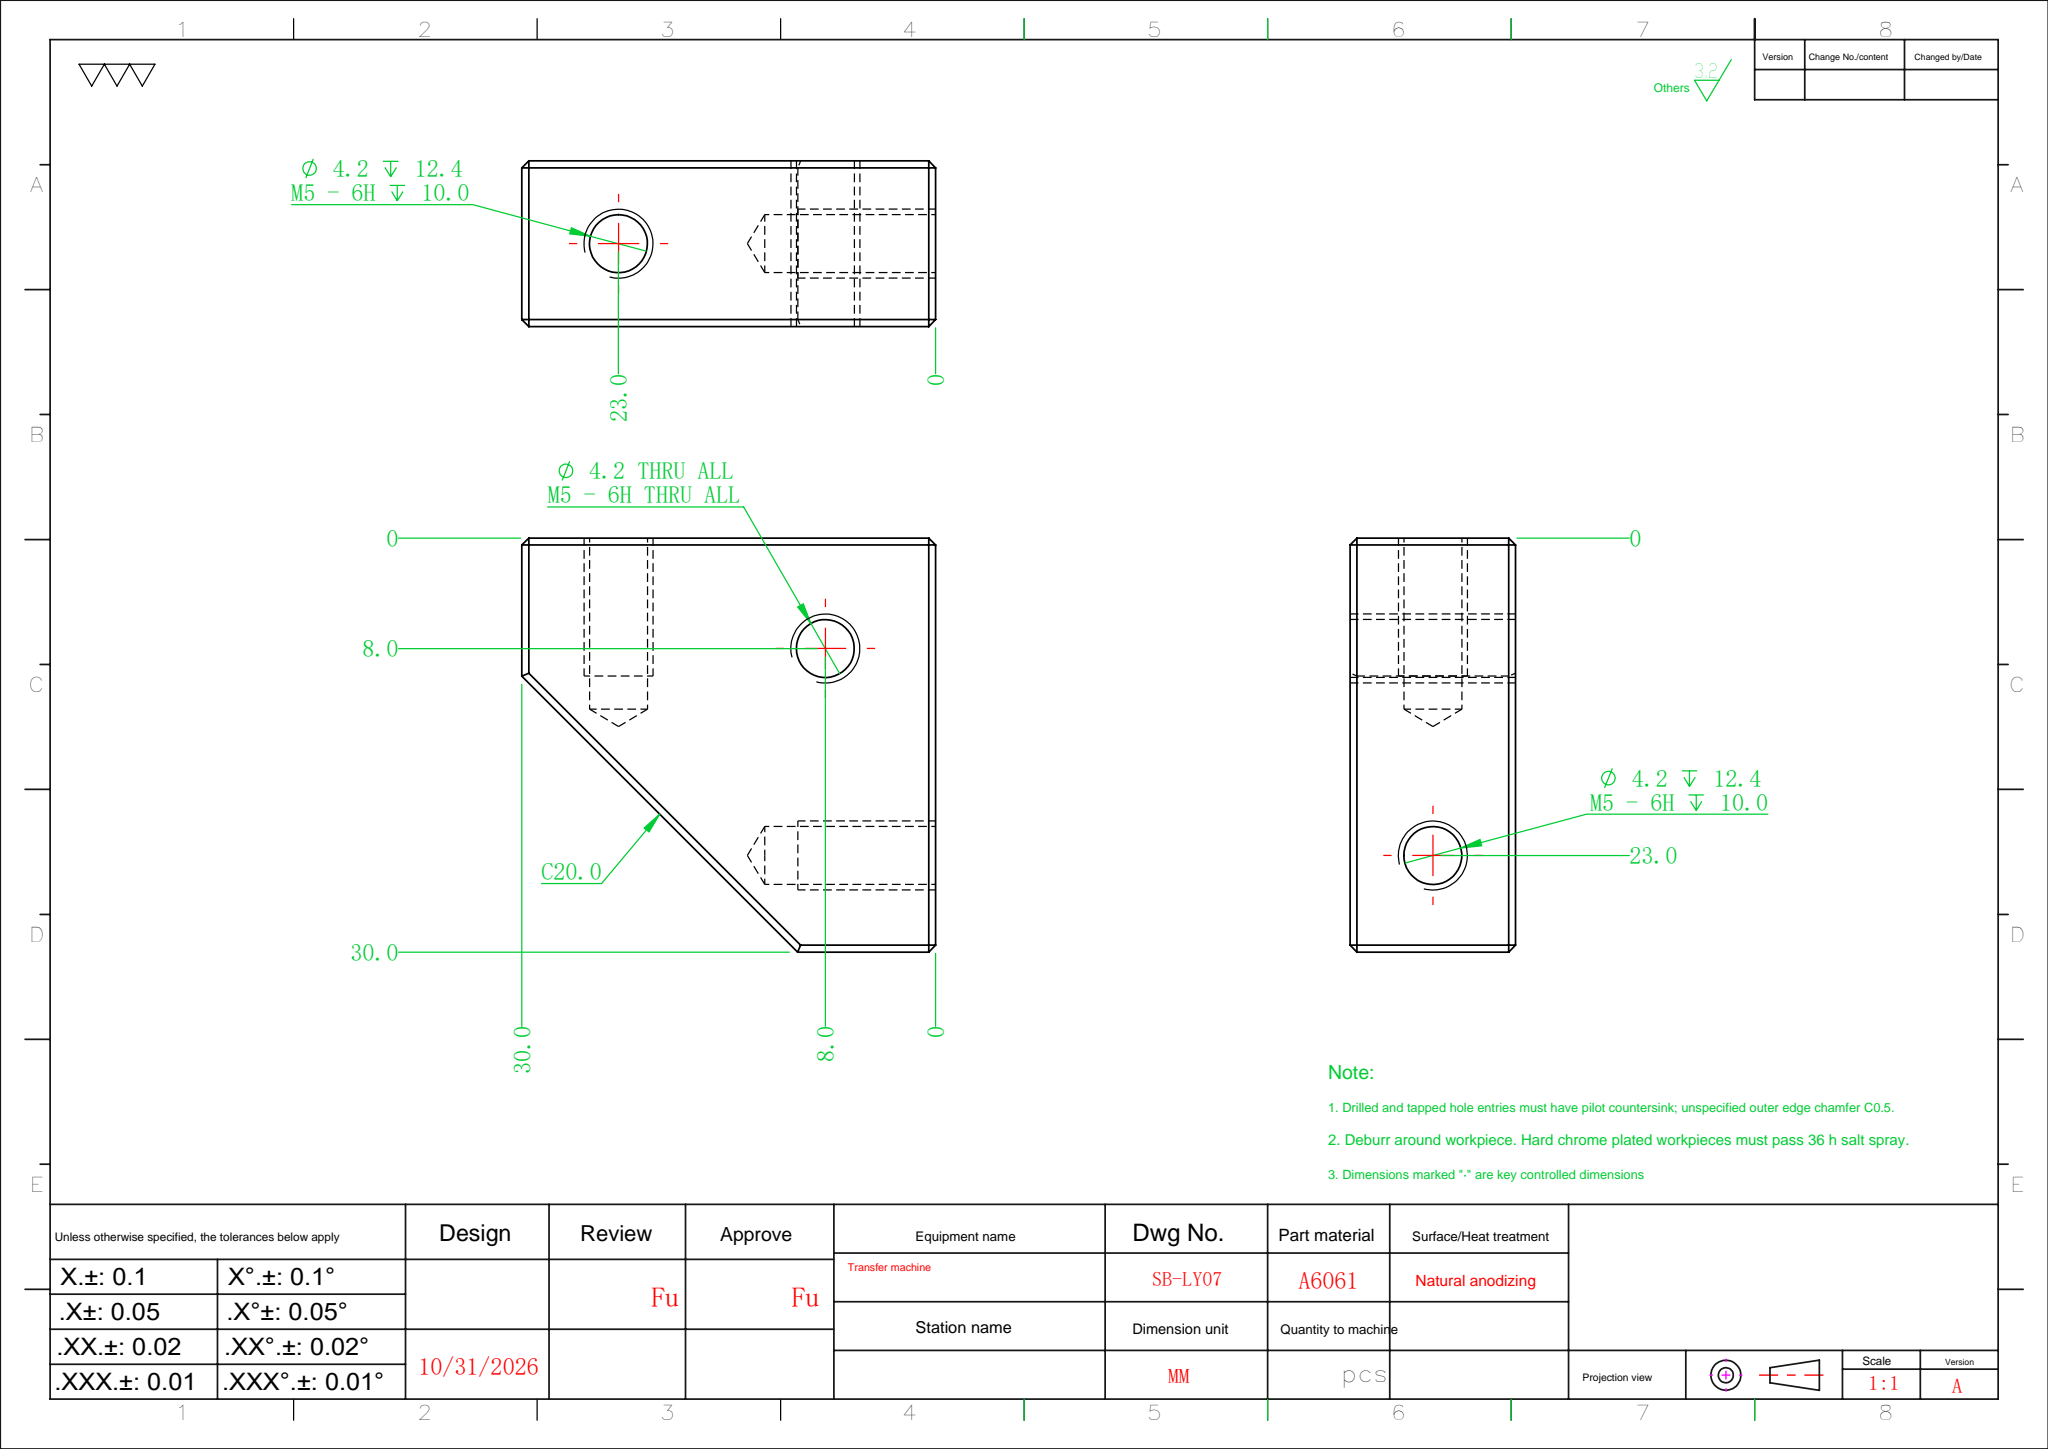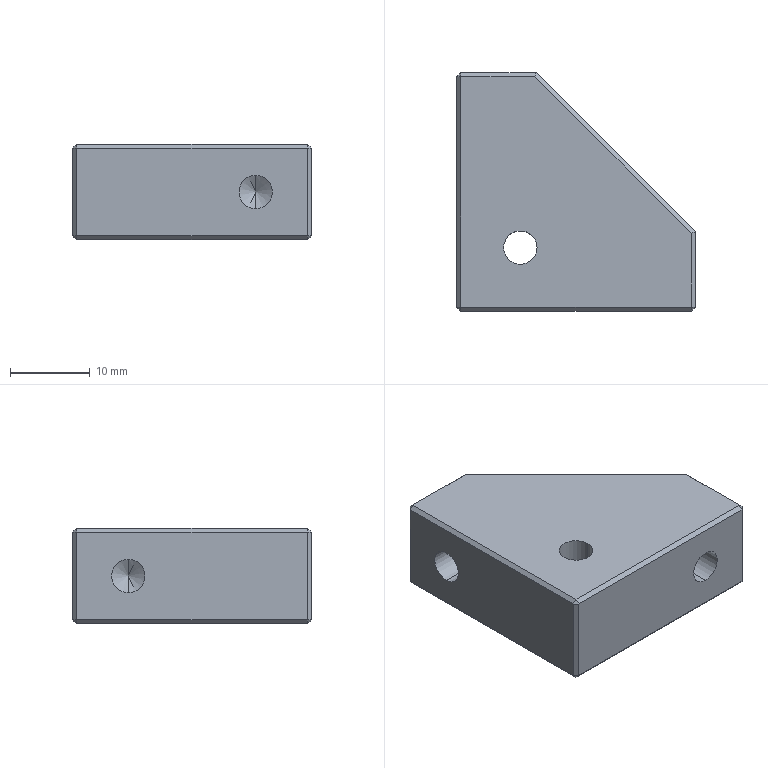Part | SolidWorks | features HoleWzd 3, Chamfer 2, Extrusion 1 | 1 solid | 36 faces | box 30 x 30 x 12 mm | volume 7848 mm3 | plane 26 | cylinder 6 | cone 4 | commonest cylinder face diameters 4.2 x6
STEP:
#1=CARTESIAN_POINT('',(-2.6,8.,3.9));
#2=VERTEX_POINT('',#1);
#3=CARTESIAN_POINT('',(-2.6,8.,8.1));
#4=VERTEX_POINT('',#3);
#5=CARTESIAN_POINT('',(-2.6,8.,6.));
#6=DIRECTION('',(-1.,0.,0.));
#7=DIRECTION('',(0.,0.,1.));
#8=AXIS2_PLACEMENT_3D('',#5,#6,#7);
#9=CIRCLE('',#8,2.1);
#10=EDGE_CURVE('',#2,#4,#9,.T.);
#11=ORIENTED_EDGE('',*,*,#10,.F.);
#12=CARTESIAN_POINT('',(-15.,8.,3.9));
#13=VERTEX_POINT('',#12);
#14=CARTESIAN_POINT('',(-15.,8.,3.9));
#15=DIRECTION('',(-1.,0.,0.));
#16=VECTOR('',#15,1000.);
#17=LINE('',#14,#16);
#18=EDGE_CURVE('',#2,#13,#17,.T.);
#19=ORIENTED_EDGE('',*,*,#18,.T.);
#20=CARTESIAN_POINT('',(-15.,8.,8.1));
#21=VERTEX_POINT('',#20);
#22=CARTESIAN_POINT('',(-15.,8.,6.));
#23=DIRECTION('',(-1.,0.,0.));
#24=DIRECTION('',(0.,0.,1.));
#25=AXIS2_PLACEMENT_3D('',#22,#23,#24);
#26=CIRCLE('',#25,2.1);
#27=EDGE_CURVE('',#13,#21,#26,.T.);
#28=ORIENTED_EDGE('',*,*,#27,.T.);
#29=CARTESIAN_POINT('',(-15.,8.,8.1));
#30=DIRECTION('',(-1.,0.,0.));
#31=VECTOR('',#30,1000.);
#32=LINE('',#29,#31);
#33=EDGE_CURVE('',#4,#21,#32,.T.);
#34=ORIENTED_EDGE('',*,*,#33,.F.);
#35=EDGE_LOOP('',(#11,#19,#28,#34));
#36=FACE_OUTER_BOUND('',#35,.T.);
#37=CARTESIAN_POINT('',(-15.,8.,6.));
#38=DIRECTION('',(-1.,0.,0.));
#39=DIRECTION('',(0.,0.,1.));
#40=AXIS2_PLACEMENT_3D('',#37,#38,#39);
#41=CYLINDRICAL_SURFACE('',#40,2.1);
#42=ADVANCED_FACE('',(#36),#41,.F.);
#43=CARTESIAN_POINT('',(-1.338,8.,6.));
#44=VERTEX_POINT('',#43);
#45=CARTESIAN_POINT('',(-2.6,8.,8.1));
#46=DIRECTION('',(-0.515,0.,0.8572));
#47=VECTOR('',#46,1000.);
#48=LINE('',#45,#47);
#49=EDGE_CURVE('',#44,#4,#48,.T.);
#50=ORIENTED_EDGE('',*,*,#49,.F.);
#51=CARTESIAN_POINT('',(-2.6,8.,3.9));
#52=DIRECTION('',(-0.515,0.,-0.8572));
#53=VECTOR('',#52,1000.);
#54=LINE('',#51,#53);
#55=EDGE_CURVE('',#44,#2,#54,.T.);
#56=ORIENTED_EDGE('',*,*,#55,.T.);
#57=ORIENTED_EDGE('',*,*,#10,.T.);
#58=EDGE_LOOP('',(#50,#56,#57));
#59=FACE_OUTER_BOUND('',#58,.T.);
#60=CARTESIAN_POINT('',(-2.6,8.,6.));
#61=DIRECTION('',(-1.,0.,0.));
#62=DIRECTION('',(0.,0.,1.));
#63=AXIS2_PLACEMENT_3D('',#60,#61,#62);
#64=CONICAL_SURFACE('',#63,2.1,1.03);
#65=ADVANCED_FACE('',(#59),#64,.F.);
#66=CARTESIAN_POINT('',(8.,-2.6,8.1));
#67=VERTEX_POINT('',#66);
#68=CARTESIAN_POINT('',(8.,-2.6,3.9));
#69=VERTEX_POINT('',#68);
#70=CARTESIAN_POINT('',(8.,-2.6,6.));
#71=DIRECTION('',(0.,-1.,0.));
#72=DIRECTION('',(0.,0.,-1.));
#73=AXIS2_PLACEMENT_3D('',#70,#71,#72);
#74=CIRCLE('',#73,2.1);
#75=EDGE_CURVE('',#67,#69,#74,.T.);
#76=ORIENTED_EDGE('',*,*,#75,.F.);
#77=CARTESIAN_POINT('',(8.,-15.,8.1));
#78=VERTEX_POINT('',#77);
#79=CARTESIAN_POINT('',(8.,-15.,8.1));
#80=DIRECTION('',(0.,-1.,0.));
#81=VECTOR('',#80,1000.);
#82=LINE('',#79,#81);
#83=EDGE_CURVE('',#67,#78,#82,.T.);
#84=ORIENTED_EDGE('',*,*,#83,.T.);
#85=CARTESIAN_POINT('',(8.,-15.,3.9));
#86=VERTEX_POINT('',#85);
#87=CARTESIAN_POINT('',(8.,-15.,6.));
#88=DIRECTION('',(0.,-1.,0.));
#89=DIRECTION('',(0.,0.,-1.));
#90=AXIS2_PLACEMENT_3D('',#87,#88,#89);
#91=CIRCLE('',#90,2.1);
#92=EDGE_CURVE('',#78,#86,#91,.T.);
#93=ORIENTED_EDGE('',*,*,#92,.T.);
#94=CARTESIAN_POINT('',(8.,-15.,3.9));
#95=DIRECTION('',(0.,-1.,0.));
#96=VECTOR('',#95,1000.);
#97=LINE('',#94,#96);
#98=EDGE_CURVE('',#69,#86,#97,.T.);
#99=ORIENTED_EDGE('',*,*,#98,.F.);
#100=EDGE_LOOP('',(#76,#84,#93,#99));
#101=FACE_OUTER_BOUND('',#100,.T.);
#102=CARTESIAN_POINT('',(8.,-15.,6.));
#103=DIRECTION('',(0.,-1.,0.));
#104=DIRECTION('',(0.,0.,-1.));
#105=AXIS2_PLACEMENT_3D('',#102,#103,#104);
#106=CYLINDRICAL_SURFACE('',#105,2.1);
#107=ADVANCED_FACE('',(#101),#106,.F.);
#108=CARTESIAN_POINT('',(8.,-1.338,6.));
#109=VERTEX_POINT('',#108);
#110=CARTESIAN_POINT('',(8.,-2.6,3.9));
#111=DIRECTION('',(0.,-0.515,-0.8572));
#112=VECTOR('',#111,1000.);
#113=LINE('',#110,#112);
#114=EDGE_CURVE('',#109,#69,#113,.T.);
#115=ORIENTED_EDGE('',*,*,#114,.F.);
#116=CARTESIAN_POINT('',(8.,-2.6,8.1));
#117=DIRECTION('',(0.,-0.515,0.8572));
#118=VECTOR('',#117,1000.);
#119=LINE('',#116,#118);
#120=EDGE_CURVE('',#109,#67,#119,.T.);
#121=ORIENTED_EDGE('',*,*,#120,.T.);
#122=ORIENTED_EDGE('',*,*,#75,.T.);
#123=EDGE_LOOP('',(#115,#121,#122));
#124=FACE_OUTER_BOUND('',#123,.T.);
#125=CARTESIAN_POINT('',(8.,-2.6,6.));
#126=DIRECTION('',(0.,-1.,0.));
#127=DIRECTION('',(0.,0.,-1.));
#128=AXIS2_PLACEMENT_3D('',#125,#126,#127);
#129=CONICAL_SURFACE('',#128,2.1,1.03);
#130=ADVANCED_FACE('',(#124),#129,.F.);
#131=CARTESIAN_POINT('',(-9.1,-7.,0.));
#132=VERTEX_POINT('',#131);
#133=CARTESIAN_POINT('',(-4.9,-7.,0.));
#134=VERTEX_POINT('',#133);
#135=CARTESIAN_POINT('',(-7.,-7.,0.));
#136=DIRECTION('',(0.,0.,1.));
#137=DIRECTION('',(1.,0.,0.));
#138=AXIS2_PLACEMENT_3D('',#135,#136,#137);
#139=CIRCLE('',#138,2.1);
#140=EDGE_CURVE('',#132,#134,#139,.T.);
#141=ORIENTED_EDGE('',*,*,#140,.F.);
#142=CARTESIAN_POINT('',(-9.1,-7.,12.));
#143=VERTEX_POINT('',#142);
#144=CARTESIAN_POINT('',(-9.1,-7.,12.));
#145=DIRECTION('',(0.,0.,1.));
#146=VECTOR('',#145,1000.);
#147=LINE('',#144,#146);
#148=EDGE_CURVE('',#132,#143,#147,.T.);
#149=ORIENTED_EDGE('',*,*,#148,.T.);
#150=CARTESIAN_POINT('',(-4.9,-7.,12.));
#151=VERTEX_POINT('',#150);
#152=CARTESIAN_POINT('',(-7.,-7.,12.));
#153=DIRECTION('',(0.,0.,1.));
#154=DIRECTION('',(1.,0.,0.));
#155=AXIS2_PLACEMENT_3D('',#152,#153,#154);
#156=CIRCLE('',#155,2.1);
#157=EDGE_CURVE('',#143,#151,#156,.T.);
#158=ORIENTED_EDGE('',*,*,#157,.T.);
#159=CARTESIAN_POINT('',(-4.9,-7.,12.));
#160=DIRECTION('',(0.,0.,1.));
#161=VECTOR('',#160,1000.);
#162=LINE('',#159,#161);
#163=EDGE_CURVE('',#134,#151,#162,.T.);
#164=ORIENTED_EDGE('',*,*,#163,.F.);
#165=EDGE_LOOP('',(#141,#149,#158,#164));
#166=FACE_OUTER_BOUND('',#165,.T.);
#167=CARTESIAN_POINT('',(-7.,-7.,12.));
#168=DIRECTION('',(0.,0.,1.));
#169=DIRECTION('',(1.,0.,0.));
#170=AXIS2_PLACEMENT_3D('',#167,#168,#169);
#171=CYLINDRICAL_SURFACE('',#170,2.1);
#172=ADVANCED_FACE('',(#166),#171,.F.);
#173=CARTESIAN_POINT('',(15.,-14.5,11.5));
#174=VERTEX_POINT('',#173);
#175=CARTESIAN_POINT('',(15.,-14.5,0.5));
#176=VERTEX_POINT('',#175);
#177=CARTESIAN_POINT('',(15.,-14.5,12.));
#178=DIRECTION('',(0.,0.,-1.));
#179=VECTOR('',#178,1000.);
#180=LINE('',#177,#179);
#181=EDGE_CURVE('',#174,#176,#180,.T.);
#182=ORIENTED_EDGE('',*,*,#181,.T.);
#183=CARTESIAN_POINT('',(15.,-5.,0.5));
#184=VERTEX_POINT('',#183);
#185=CARTESIAN_POINT('',(15.,-5.,0.5));
#186=DIRECTION('',(0.,1.,0.));
#187=VECTOR('',#186,1000.);
#188=LINE('',#185,#187);
#189=EDGE_CURVE('',#176,#184,#188,.T.);
#190=ORIENTED_EDGE('',*,*,#189,.T.);
#191=CARTESIAN_POINT('',(15.,-5.,11.5));
#192=VERTEX_POINT('',#191);
#193=CARTESIAN_POINT('',(15.,-5.,12.));
#194=DIRECTION('',(0.,0.,1.));
#195=VECTOR('',#194,1000.);
#196=LINE('',#193,#195);
#197=EDGE_CURVE('',#184,#192,#196,.T.);
#198=ORIENTED_EDGE('',*,*,#197,.T.);
#199=CARTESIAN_POINT('',(15.,-15.,11.5));
#200=DIRECTION('',(0.,-1.,0.));
#201=VECTOR('',#200,1000.);
#202=LINE('',#199,#201);
#203=EDGE_CURVE('',#192,#174,#202,.T.);
#204=ORIENTED_EDGE('',*,*,#203,.T.);
#205=EDGE_LOOP('',(#182,#190,#198,#204));
#206=FACE_OUTER_BOUND('',#205,.T.);
#207=CARTESIAN_POINT('',(15.,-15.,12.));
#208=DIRECTION('',(-1.,0.,0.));
#209=DIRECTION('',(0.,0.,1.));
#210=AXIS2_PLACEMENT_3D('',#207,#208,#209);
#211=PLANE('',#210);
#212=ADVANCED_FACE('',(#206),#211,.F.);
#213=CARTESIAN_POINT('',(-5.,15.,11.5));
#214=VERTEX_POINT('',#213);
#215=CARTESIAN_POINT('',(-5.,15.,0.5));
#216=VERTEX_POINT('',#215);
#217=CARTESIAN_POINT('',(-5.,15.,12.));
#218=DIRECTION('',(0.,0.,-1.));
#219=VECTOR('',#218,1000.);
#220=LINE('',#217,#219);
#221=EDGE_CURVE('',#214,#216,#220,.T.);
#222=ORIENTED_EDGE('',*,*,#221,.T.);
#223=CARTESIAN_POINT('',(-14.5,15.,0.5));
#224=VERTEX_POINT('',#223);
#225=CARTESIAN_POINT('',(-15.,15.,0.5));
#226=DIRECTION('',(-1.,0.,0.));
#227=VECTOR('',#226,1000.);
#228=LINE('',#225,#227);
#229=EDGE_CURVE('',#216,#224,#228,.T.);
#230=ORIENTED_EDGE('',*,*,#229,.T.);
#231=CARTESIAN_POINT('',(-14.5,15.,11.5));
#232=VERTEX_POINT('',#231);
#233=CARTESIAN_POINT('',(-14.5,15.,12.));
#234=DIRECTION('',(0.,0.,1.));
#235=VECTOR('',#234,1000.);
#236=LINE('',#233,#235);
#237=EDGE_CURVE('',#224,#232,#236,.T.);
#238=ORIENTED_EDGE('',*,*,#237,.T.);
#239=CARTESIAN_POINT('',(-15.,15.,11.5));
#240=DIRECTION('',(1.,0.,0.));
#241=VECTOR('',#240,1000.);
#242=LINE('',#239,#241);
#243=EDGE_CURVE('',#232,#214,#242,.T.);
#244=ORIENTED_EDGE('',*,*,#243,.T.);
#245=EDGE_LOOP('',(#222,#230,#238,#244));
#246=FACE_OUTER_BOUND('',#245,.T.);
#247=CARTESIAN_POINT('',(-15.,15.,12.));
#248=DIRECTION('',(0.,-1.,0.));
#249=DIRECTION('',(0.,0.,-1.));
#250=AXIS2_PLACEMENT_3D('',#247,#248,#249);
#251=PLANE('',#250);
#252=ADVANCED_FACE('',(#246),#251,.F.);
#253=CARTESIAN_POINT('',(-15.,-14.5,11.5));
#254=VERTEX_POINT('',#253);
#255=CARTESIAN_POINT('',(-15.,14.5,11.5));
#256=VERTEX_POINT('',#255);
#257=CARTESIAN_POINT('',(-15.,-15.,11.5));
#258=DIRECTION('',(0.,1.,0.));
#259=VECTOR('',#258,1000.);
#260=LINE('',#257,#259);
#261=EDGE_CURVE('',#254,#256,#260,.T.);
#262=ORIENTED_EDGE('',*,*,#261,.T.);
#263=CARTESIAN_POINT('',(-15.,14.5,0.5));
#264=VERTEX_POINT('',#263);
#265=CARTESIAN_POINT('',(-15.,14.5,12.));
#266=DIRECTION('',(0.,0.,-1.));
#267=VECTOR('',#266,1000.);
#268=LINE('',#265,#267);
#269=EDGE_CURVE('',#256,#264,#268,.T.);
#270=ORIENTED_EDGE('',*,*,#269,.T.);
#271=CARTESIAN_POINT('',(-15.,-14.5,0.5));
#272=VERTEX_POINT('',#271);
#273=CARTESIAN_POINT('',(-15.,-15.,0.5));
#274=DIRECTION('',(0.,-1.,0.));
#275=VECTOR('',#274,1000.);
#276=LINE('',#273,#275);
#277=EDGE_CURVE('',#264,#272,#276,.T.);
#278=ORIENTED_EDGE('',*,*,#277,.T.);
#279=CARTESIAN_POINT('',(-15.,-14.5,12.));
#280=DIRECTION('',(0.,0.,1.));
#281=VECTOR('',#280,1000.);
#282=LINE('',#279,#281);
#283=EDGE_CURVE('',#272,#254,#282,.T.);
#284=ORIENTED_EDGE('',*,*,#283,.T.);
#285=EDGE_LOOP('',(#262,#270,#278,#284));
#286=FACE_OUTER_BOUND('',#285,.T.);
#287=CARTESIAN_POINT('',(-15.,8.,6.));
#288=DIRECTION('',(-1.,0.,0.));
#289=DIRECTION('',(0.,0.,1.));
#290=AXIS2_PLACEMENT_3D('',#287,#288,#289);
#291=CIRCLE('',#290,2.1);
#292=EDGE_CURVE('',#21,#13,#291,.T.);
#293=ORIENTED_EDGE('',*,*,#292,.F.);
#294=ORIENTED_EDGE('',*,*,#27,.F.);
#295=EDGE_LOOP('',(#293,#294));
#296=FACE_BOUND('',#295,.T.);
#297=CARTESIAN_POINT('',(-15.,-15.,12.));
#298=DIRECTION('',(1.,0.,0.));
#299=DIRECTION('',(0.,0.,-1.));
#300=AXIS2_PLACEMENT_3D('',#297,#298,#299);
#301=PLANE('',#300);
#302=ADVANCED_FACE('',(#286,#296),#301,.F.);
#303=CARTESIAN_POINT('',(14.5,-15.,0.5));
#304=VERTEX_POINT('',#303);
#305=CARTESIAN_POINT('',(14.5,-15.,11.5));
#306=VERTEX_POINT('',#305);
#307=CARTESIAN_POINT('',(14.5,-15.,12.));
#308=DIRECTION('',(0.,0.,1.));
#309=VECTOR('',#308,1000.);
#310=LINE('',#307,#309);
#311=EDGE_CURVE('',#304,#306,#310,.T.);
#312=ORIENTED_EDGE('',*,*,#311,.T.);
#313=CARTESIAN_POINT('',(-14.5,-15.,11.5));
#314=VERTEX_POINT('',#313);
#315=CARTESIAN_POINT('',(-15.,-15.,11.5));
#316=DIRECTION('',(-1.,0.,0.));
#317=VECTOR('',#316,1000.);
#318=LINE('',#315,#317);
#319=EDGE_CURVE('',#306,#314,#318,.T.);
#320=ORIENTED_EDGE('',*,*,#319,.T.);
#321=CARTESIAN_POINT('',(-14.5,-15.,0.5));
#322=VERTEX_POINT('',#321);
#323=CARTESIAN_POINT('',(-14.5,-15.,12.));
#324=DIRECTION('',(0.,0.,-1.));
#325=VECTOR('',#324,1000.);
#326=LINE('',#323,#325);
#327=EDGE_CURVE('',#314,#322,#326,.T.);
#328=ORIENTED_EDGE('',*,*,#327,.T.);
#329=CARTESIAN_POINT('',(15.,-15.,0.5));
#330=DIRECTION('',(1.,0.,0.));
#331=VECTOR('',#330,1000.);
#332=LINE('',#329,#331);
#333=EDGE_CURVE('',#322,#304,#332,.T.);
#334=ORIENTED_EDGE('',*,*,#333,.T.);
#335=EDGE_LOOP('',(#312,#320,#328,#334));
#336=FACE_OUTER_BOUND('',#335,.T.);
#337=CARTESIAN_POINT('',(8.,-15.,6.));
#338=DIRECTION('',(0.,-1.,0.));
#339=DIRECTION('',(0.,0.,-1.));
#340=AXIS2_PLACEMENT_3D('',#337,#338,#339);
#341=CIRCLE('',#340,2.1);
#342=EDGE_CURVE('',#86,#78,#341,.T.);
#343=ORIENTED_EDGE('',*,*,#342,.F.);
#344=ORIENTED_EDGE('',*,*,#92,.F.);
#345=EDGE_LOOP('',(#343,#344));
#346=FACE_BOUND('',#345,.T.);
#347=CARTESIAN_POINT('',(-15.,-15.,12.));
#348=DIRECTION('',(0.,1.,0.));
#349=DIRECTION('',(0.,0.,1.));
#350=AXIS2_PLACEMENT_3D('',#347,#348,#349);
#351=PLANE('',#350);
#352=ADVANCED_FACE('',(#336,#346),#351,.F.);
#353=CARTESIAN_POINT('',(14.5,-5.207,12.));
#354=VERTEX_POINT('',#353);
#355=CARTESIAN_POINT('',(-5.207,14.5,12.));
#356=VERTEX_POINT('',#355);
#357=CARTESIAN_POINT('',(-5.354,14.646,12.));
#358=DIRECTION('',(-0.7071,0.7071,0.));
#359=VECTOR('',#358,1000.);
#360=LINE('',#357,#359);
#361=EDGE_CURVE('',#354,#356,#360,.T.);
#362=ORIENTED_EDGE('',*,*,#361,.T.);
#363=CARTESIAN_POINT('',(-14.5,14.5,12.));
#364=VERTEX_POINT('',#363);
#365=CARTESIAN_POINT('',(0.,14.5,12.));
#366=DIRECTION('',(-1.,0.,0.));
#367=VECTOR('',#366,1000.);
#368=LINE('',#365,#367);
#369=EDGE_CURVE('',#356,#364,#368,.T.);
#370=ORIENTED_EDGE('',*,*,#369,.T.);
#371=CARTESIAN_POINT('',(-14.5,-14.5,12.));
#372=VERTEX_POINT('',#371);
#373=CARTESIAN_POINT('',(-14.5,0.,12.));
#374=DIRECTION('',(0.,-1.,0.));
#375=VECTOR('',#374,1000.);
#376=LINE('',#373,#375);
#377=EDGE_CURVE('',#364,#372,#376,.T.);
#378=ORIENTED_EDGE('',*,*,#377,.T.);
#379=CARTESIAN_POINT('',(14.5,-14.5,12.));
#380=VERTEX_POINT('',#379);
#381=CARTESIAN_POINT('',(0.,-14.5,12.));
#382=DIRECTION('',(1.,0.,0.));
#383=VECTOR('',#382,1000.);
#384=LINE('',#381,#383);
#385=EDGE_CURVE('',#372,#380,#384,.T.);
#386=ORIENTED_EDGE('',*,*,#385,.T.);
#387=CARTESIAN_POINT('',(14.5,0.,12.));
#388=DIRECTION('',(0.,1.,0.));
#389=VECTOR('',#388,1000.);
#390=LINE('',#387,#389);
#391=EDGE_CURVE('',#380,#354,#390,.T.);
#392=ORIENTED_EDGE('',*,*,#391,.T.);
#393=EDGE_LOOP('',(#362,#370,#378,#386,#392));
#394=FACE_OUTER_BOUND('',#393,.T.);
#395=CARTESIAN_POINT('',(-7.,-7.,12.));
#396=DIRECTION('',(0.,0.,1.));
#397=DIRECTION('',(1.,0.,0.));
#398=AXIS2_PLACEMENT_3D('',#395,#396,#397);
#399=CIRCLE('',#398,2.1);
#400=EDGE_CURVE('',#151,#143,#399,.T.);
#401=ORIENTED_EDGE('',*,*,#400,.F.);
#402=ORIENTED_EDGE('',*,*,#157,.F.);
#403=EDGE_LOOP('',(#401,#402));
#404=FACE_BOUND('',#403,.T.);
#405=CARTESIAN_POINT('',(0.,0.,12.));
#406=DIRECTION('',(0.,0.,-1.));
#407=DIRECTION('',(-1.,0.,0.));
#408=AXIS2_PLACEMENT_3D('',#405,#406,#407);
#409=PLANE('',#408);
#410=ADVANCED_FACE('',(#394,#404),#409,.F.);
#411=CARTESIAN_POINT('',(-5.207,14.5,0.));
#412=VERTEX_POINT('',#411);
#413=CARTESIAN_POINT('',(14.5,-5.207,0.));
#414=VERTEX_POINT('',#413);
#415=CARTESIAN_POINT('',(4.646,4.646,0.));
#416=DIRECTION('',(0.7071,-0.7071,0.));
#417=VECTOR('',#416,1000.);
#418=LINE('',#415,#417);
#419=EDGE_CURVE('',#412,#414,#418,.T.);
#420=ORIENTED_EDGE('',*,*,#419,.T.);
#421=CARTESIAN_POINT('',(14.5,-14.5,0.));
#422=VERTEX_POINT('',#421);
#423=CARTESIAN_POINT('',(14.5,-15.,0.));
#424=DIRECTION('',(0.,-1.,0.));
#425=VECTOR('',#424,1000.);
#426=LINE('',#423,#425);
#427=EDGE_CURVE('',#414,#422,#426,.T.);
#428=ORIENTED_EDGE('',*,*,#427,.T.);
#429=CARTESIAN_POINT('',(-14.5,-14.5,0.));
#430=VERTEX_POINT('',#429);
#431=CARTESIAN_POINT('',(-15.,-14.5,0.));
#432=DIRECTION('',(-1.,0.,0.));
#433=VECTOR('',#432,1000.);
#434=LINE('',#431,#433);
#435=EDGE_CURVE('',#422,#430,#434,.T.);
#436=ORIENTED_EDGE('',*,*,#435,.T.);
#437=CARTESIAN_POINT('',(-14.5,14.5,0.));
#438=VERTEX_POINT('',#437);
#439=CARTESIAN_POINT('',(-14.5,15.,0.));
#440=DIRECTION('',(0.,1.,0.));
#441=VECTOR('',#440,1000.);
#442=LINE('',#439,#441);
#443=EDGE_CURVE('',#430,#438,#442,.T.);
#444=ORIENTED_EDGE('',*,*,#443,.T.);
#445=CARTESIAN_POINT('',(-5.,14.5,0.));
#446=DIRECTION('',(1.,0.,0.));
#447=VECTOR('',#446,1000.);
#448=LINE('',#445,#447);
#449=EDGE_CURVE('',#438,#412,#448,.T.);
#450=ORIENTED_EDGE('',*,*,#449,.T.);
#451=EDGE_LOOP('',(#420,#428,#436,#444,#450));
#452=FACE_OUTER_BOUND('',#451,.T.);
#453=CARTESIAN_POINT('',(-7.,-7.,0.));
#454=DIRECTION('',(0.,0.,1.));
#455=DIRECTION('',(1.,0.,0.));
#456=AXIS2_PLACEMENT_3D('',#453,#454,#455);
#457=CIRCLE('',#456,2.1);
#458=EDGE_CURVE('',#134,#132,#457,.T.);
#459=ORIENTED_EDGE('',*,*,#458,.T.);
#460=ORIENTED_EDGE('',*,*,#140,.T.);
#461=EDGE_LOOP('',(#459,#460));
#462=FACE_BOUND('',#461,.T.);
#463=CARTESIAN_POINT('',(0.,0.,0.));
#464=DIRECTION('',(0.,0.,-1.));
#465=DIRECTION('',(-1.,0.,0.));
#466=AXIS2_PLACEMENT_3D('',#463,#464,#465);
#467=PLANE('',#466);
#468=ADVANCED_FACE('',(#452,#462),#467,.T.);
#469=ORIENTED_EDGE('',*,*,#197,.F.);
#470=CARTESIAN_POINT('',(-5.,15.,0.5));
#471=DIRECTION('',(-0.7071,0.7071,0.));
#472=VECTOR('',#471,1000.);
#473=LINE('',#470,#472);
#474=EDGE_CURVE('',#184,#216,#473,.T.);
#475=ORIENTED_EDGE('',*,*,#474,.T.);
#476=ORIENTED_EDGE('',*,*,#221,.F.);
#477=CARTESIAN_POINT('',(15.,-5.,11.5));
#478=DIRECTION('',(0.7071,-0.7071,0.));
#479=VECTOR('',#478,1000.);
#480=LINE('',#477,#479);
#481=EDGE_CURVE('',#214,#192,#480,.T.);
#482=ORIENTED_EDGE('',*,*,#481,.T.);
#483=EDGE_LOOP('',(#469,#475,#476,#482));
#484=FACE_OUTER_BOUND('',#483,.T.);
#485=CARTESIAN_POINT('',(-5.,15.,12.));
#486=DIRECTION('',(-0.7071,-0.7071,0.));
#487=DIRECTION('',(0.,0.,-1.));
#488=AXIS2_PLACEMENT_3D('',#485,#486,#487);
#489=PLANE('',#488);
#490=ADVANCED_FACE('',(#484),#489,.F.);
#491=ORIENTED_EDGE('',*,*,#148,.F.);
#492=ORIENTED_EDGE('',*,*,#458,.F.);
#493=ORIENTED_EDGE('',*,*,#163,.T.);
#494=ORIENTED_EDGE('',*,*,#400,.T.);
#495=EDGE_LOOP('',(#491,#492,#493,#494));
#496=FACE_OUTER_BOUND('',#495,.T.);
#497=CARTESIAN_POINT('',(-7.,-7.,12.));
#498=DIRECTION('',(0.,0.,1.));
#499=DIRECTION('',(1.,0.,0.));
#500=AXIS2_PLACEMENT_3D('',#497,#498,#499);
#501=CYLINDRICAL_SURFACE('',#500,2.1);
#502=ADVANCED_FACE('',(#496),#501,.F.);
#503=ORIENTED_EDGE('',*,*,#120,.F.);
#504=ORIENTED_EDGE('',*,*,#114,.T.);
#505=CARTESIAN_POINT('',(8.,-2.6,6.));
#506=DIRECTION('',(0.,-1.,0.));
#507=DIRECTION('',(0.,0.,-1.));
#508=AXIS2_PLACEMENT_3D('',#505,#506,#507);
#509=CIRCLE('',#508,2.1);
#510=EDGE_CURVE('',#69,#67,#509,.T.);
#511=ORIENTED_EDGE('',*,*,#510,.T.);
#512=EDGE_LOOP('',(#503,#504,#511));
#513=FACE_OUTER_BOUND('',#512,.T.);
#514=CARTESIAN_POINT('',(8.,-2.6,6.));
#515=DIRECTION('',(0.,-1.,0.));
#516=DIRECTION('',(0.,0.,-1.));
#517=AXIS2_PLACEMENT_3D('',#514,#515,#516);
#518=CONICAL_SURFACE('',#517,2.1,1.03);
#519=ADVANCED_FACE('',(#513),#518,.F.);
#520=ORIENTED_EDGE('',*,*,#83,.F.);
#521=ORIENTED_EDGE('',*,*,#510,.F.);
#522=ORIENTED_EDGE('',*,*,#98,.T.);
#523=ORIENTED_EDGE('',*,*,#342,.T.);
#524=EDGE_LOOP('',(#520,#521,#522,#523));
#525=FACE_OUTER_BOUND('',#524,.T.);
#526=CARTESIAN_POINT('',(8.,-15.,6.));
#527=DIRECTION('',(0.,-1.,0.));
#528=DIRECTION('',(0.,0.,-1.));
#529=AXIS2_PLACEMENT_3D('',#526,#527,#528);
#530=CYLINDRICAL_SURFACE('',#529,2.1);
#531=ADVANCED_FACE('',(#525),#530,.F.);
#532=ORIENTED_EDGE('',*,*,#55,.F.);
#533=ORIENTED_EDGE('',*,*,#49,.T.);
#534=CARTESIAN_POINT('',(-2.6,8.,6.));
#535=DIRECTION('',(-1.,0.,0.));
#536=DIRECTION('',(0.,0.,1.));
#537=AXIS2_PLACEMENT_3D('',#534,#535,#536);
#538=CIRCLE('',#537,2.1);
#539=EDGE_CURVE('',#4,#2,#538,.T.);
#540=ORIENTED_EDGE('',*,*,#539,.T.);
#541=EDGE_LOOP('',(#532,#533,#540));
#542=FACE_OUTER_BOUND('',#541,.T.);
#543=CARTESIAN_POINT('',(-2.6,8.,6.));
#544=DIRECTION('',(-1.,0.,0.));
#545=DIRECTION('',(0.,0.,1.));
#546=AXIS2_PLACEMENT_3D('',#543,#544,#545);
#547=CONICAL_SURFACE('',#546,2.1,1.03);
#548=ADVANCED_FACE('',(#542),#547,.F.);
#549=ORIENTED_EDGE('',*,*,#18,.F.);
#550=ORIENTED_EDGE('',*,*,#539,.F.);
#551=ORIENTED_EDGE('',*,*,#33,.T.);
#552=ORIENTED_EDGE('',*,*,#292,.T.);
#553=EDGE_LOOP('',(#549,#550,#551,#552));
#554=FACE_OUTER_BOUND('',#553,.T.);
#555=CARTESIAN_POINT('',(-15.,8.,6.));
#556=DIRECTION('',(-1.,0.,0.));
#557=DIRECTION('',(0.,0.,1.));
#558=AXIS2_PLACEMENT_3D('',#555,#556,#557);
#559=CYLINDRICAL_SURFACE('',#558,2.1);
#560=ADVANCED_FACE('',(#554),#559,.F.);
#561=CARTESIAN_POINT('',(-14.5,14.5,12.));
#562=DIRECTION('',(0.,0.7071,-0.7071));
#563=VECTOR('',#562,1000.);
#564=LINE('',#561,#563);
#565=EDGE_CURVE('',#364,#232,#564,.T.);
#566=ORIENTED_EDGE('',*,*,#565,.F.);
#567=ORIENTED_EDGE('',*,*,#369,.F.);
#568=CARTESIAN_POINT('',(-6.308,11.842,14.658));
#569=DIRECTION('',(-0.2811,-0.6786,0.6786));
#570=VECTOR('',#569,1000.);
#571=LINE('',#568,#570);
#572=EDGE_CURVE('',#214,#356,#571,.T.);
#573=ORIENTED_EDGE('',*,*,#572,.F.);
#574=ORIENTED_EDGE('',*,*,#243,.F.);
#575=EDGE_LOOP('',(#566,#567,#573,#574));
#576=FACE_OUTER_BOUND('',#575,.T.);
#577=CARTESIAN_POINT('',(0.,14.5,12.));
#578=DIRECTION('',(0.,-0.7071,-0.7071));
#579=DIRECTION('',(-1.,0.,0.));
#580=AXIS2_PLACEMENT_3D('',#577,#578,#579);
#581=PLANE('',#580);
#582=ADVANCED_FACE('',(#576),#581,.F.);
#583=CARTESIAN_POINT('',(-14.75,-14.5,11.75));
#584=DIRECTION('',(-0.7071,0.,-0.7071));
#585=VECTOR('',#584,1000.);
#586=LINE('',#583,#585);
#587=EDGE_CURVE('',#372,#254,#586,.T.);
#588=ORIENTED_EDGE('',*,*,#587,.F.);
#589=ORIENTED_EDGE('',*,*,#377,.F.);
#590=CARTESIAN_POINT('',(-14.5,14.5,12.));
#591=DIRECTION('',(0.7071,0.,0.7071));
#592=VECTOR('',#591,1000.);
#593=LINE('',#590,#592);
#594=EDGE_CURVE('',#256,#364,#593,.T.);
#595=ORIENTED_EDGE('',*,*,#594,.F.);
#596=ORIENTED_EDGE('',*,*,#261,.F.);
#597=EDGE_LOOP('',(#588,#589,#595,#596));
#598=FACE_OUTER_BOUND('',#597,.T.);
#599=CARTESIAN_POINT('',(-14.5,0.,12.));
#600=DIRECTION('',(0.7071,0.,-0.7071));
#601=DIRECTION('',(0.,-1.,0.));
#602=AXIS2_PLACEMENT_3D('',#599,#600,#601);
#603=PLANE('',#602);
#604=ADVANCED_FACE('',(#598),#603,.F.);
#605=CARTESIAN_POINT('',(-14.5,-15.,11.5));
#606=DIRECTION('',(0.,-0.7071,-0.7071));
#607=VECTOR('',#606,1000.);
#608=LINE('',#605,#607);
#609=EDGE_CURVE('',#372,#314,#608,.T.);
#610=ORIENTED_EDGE('',*,*,#609,.F.);
#611=ORIENTED_EDGE('',*,*,#587,.T.);
#612=CARTESIAN_POINT('',(-14.5,-15.,11.5));
#613=DIRECTION('',(-0.7071,0.7071,0.));
#614=VECTOR('',#613,1000.);
#615=LINE('',#612,#614);
#616=EDGE_CURVE('',#314,#254,#615,.T.);
#617=ORIENTED_EDGE('',*,*,#616,.F.);
#618=EDGE_LOOP('',(#610,#611,#617));
#619=FACE_OUTER_BOUND('',#618,.T.);
#620=CARTESIAN_POINT('',(-14.5,-15.,11.5));
#621=DIRECTION('',(-0.5774,-0.5774,0.5774));
#622=DIRECTION('',(0.7071,0.,0.7071));
#623=AXIS2_PLACEMENT_3D('',#620,#621,#622);
#624=PLANE('',#623);
#625=ADVANCED_FACE('',(#619),#624,.T.);
#626=ORIENTED_EDGE('',*,*,#572,.T.);
#627=ORIENTED_EDGE('',*,*,#361,.F.);
#628=CARTESIAN_POINT('',(15.493,-4.796,11.007));
#629=DIRECTION('',(-0.6786,-0.2811,0.6786));
#630=VECTOR('',#629,1000.);
#631=LINE('',#628,#630);
#632=EDGE_CURVE('',#192,#354,#631,.T.);
#633=ORIENTED_EDGE('',*,*,#632,.F.);
#634=ORIENTED_EDGE('',*,*,#481,.F.);
#635=EDGE_LOOP('',(#626,#627,#633,#634));
#636=FACE_OUTER_BOUND('',#635,.T.);
#637=CARTESIAN_POINT('',(4.646,4.646,12.));
#638=DIRECTION('',(-0.5,-0.5,-0.7071));
#639=DIRECTION('',(-0.7071,0.7071,0.));
#640=AXIS2_PLACEMENT_3D('',#637,#638,#639);
#641=PLANE('',#640);
#642=ADVANCED_FACE('',(#636),#641,.F.);
#643=ORIENTED_EDGE('',*,*,#594,.T.);
#644=ORIENTED_EDGE('',*,*,#565,.T.);
#645=CARTESIAN_POINT('',(-14.75,14.75,11.5));
#646=DIRECTION('',(0.7071,0.7071,0.));
#647=VECTOR('',#646,1000.);
#648=LINE('',#645,#647);
#649=EDGE_CURVE('',#256,#232,#648,.T.);
#650=ORIENTED_EDGE('',*,*,#649,.F.);
#651=EDGE_LOOP('',(#643,#644,#650));
#652=FACE_OUTER_BOUND('',#651,.T.);
#653=CARTESIAN_POINT('',(-14.5,14.5,12.));
#654=DIRECTION('',(-0.5774,0.5774,0.5774));
#655=DIRECTION('',(0.7071,0.,0.7071));
#656=AXIS2_PLACEMENT_3D('',#653,#654,#655);
#657=PLANE('',#656);
#658=ADVANCED_FACE('',(#652),#657,.T.);
#659=ORIENTED_EDGE('',*,*,#616,.T.);
#660=ORIENTED_EDGE('',*,*,#283,.F.);
#661=CARTESIAN_POINT('',(-14.75,-14.75,0.5));
#662=DIRECTION('',(-0.7071,0.7071,0.));
#663=VECTOR('',#662,1000.);
#664=LINE('',#661,#663);
#665=EDGE_CURVE('',#322,#272,#664,.T.);
#666=ORIENTED_EDGE('',*,*,#665,.F.);
#667=ORIENTED_EDGE('',*,*,#327,.F.);
#668=EDGE_LOOP('',(#659,#660,#666,#667));
#669=FACE_OUTER_BOUND('',#668,.T.);
#670=CARTESIAN_POINT('',(-14.5,-15.,12.));
#671=DIRECTION('',(0.7071,0.7071,0.));
#672=DIRECTION('',(0.,0.,-1.));
#673=AXIS2_PLACEMENT_3D('',#670,#671,#672);
#674=PLANE('',#673);
#675=ADVANCED_FACE('',(#669),#674,.F.);
#676=ORIENTED_EDGE('',*,*,#609,.T.);
#677=ORIENTED_EDGE('',*,*,#319,.F.);
#678=CARTESIAN_POINT('',(14.5,-14.75,11.75));
#679=DIRECTION('',(0.,-0.7071,-0.7071));
#680=VECTOR('',#679,1000.);
#681=LINE('',#678,#680);
#682=EDGE_CURVE('',#380,#306,#681,.T.);
#683=ORIENTED_EDGE('',*,*,#682,.F.);
#684=ORIENTED_EDGE('',*,*,#385,.F.);
#685=EDGE_LOOP('',(#676,#677,#683,#684));
#686=FACE_OUTER_BOUND('',#685,.T.);
#687=CARTESIAN_POINT('',(0.,-14.5,12.));
#688=DIRECTION('',(0.,0.7071,-0.7071));
#689=DIRECTION('',(1.,0.,0.));
#690=AXIS2_PLACEMENT_3D('',#687,#688,#689);
#691=PLANE('',#690);
#692=ADVANCED_FACE('',(#686),#691,.F.);
#693=ORIENTED_EDGE('',*,*,#632,.T.);
#694=ORIENTED_EDGE('',*,*,#391,.F.);
#695=CARTESIAN_POINT('',(15.,-14.5,11.5));
#696=DIRECTION('',(-0.7071,0.,0.7071));
#697=VECTOR('',#696,1000.);
#698=LINE('',#695,#697);
#699=EDGE_CURVE('',#174,#380,#698,.T.);
#700=ORIENTED_EDGE('',*,*,#699,.F.);
#701=ORIENTED_EDGE('',*,*,#203,.F.);
#702=EDGE_LOOP('',(#693,#694,#700,#701));
#703=FACE_OUTER_BOUND('',#702,.T.);
#704=CARTESIAN_POINT('',(14.5,0.,12.));
#705=DIRECTION('',(-0.7071,0.,-0.7071));
#706=DIRECTION('',(0.,1.,0.));
#707=AXIS2_PLACEMENT_3D('',#704,#705,#706);
#708=PLANE('',#707);
#709=ADVANCED_FACE('',(#703),#708,.F.);
#710=ORIENTED_EDGE('',*,*,#649,.T.);
#711=ORIENTED_EDGE('',*,*,#237,.F.);
#712=CARTESIAN_POINT('',(-14.5,15.,0.5));
#713=DIRECTION('',(0.7071,0.7071,0.));
#714=VECTOR('',#713,1000.);
#715=LINE('',#712,#714);
#716=EDGE_CURVE('',#264,#224,#715,.T.);
#717=ORIENTED_EDGE('',*,*,#716,.F.);
#718=ORIENTED_EDGE('',*,*,#269,.F.);
#719=EDGE_LOOP('',(#710,#711,#717,#718));
#720=FACE_OUTER_BOUND('',#719,.T.);
#721=CARTESIAN_POINT('',(-15.,14.5,12.));
#722=DIRECTION('',(0.7071,-0.7071,0.));
#723=DIRECTION('',(0.,0.,-1.));
#724=AXIS2_PLACEMENT_3D('',#721,#722,#723);
#725=PLANE('',#724);
#726=ADVANCED_FACE('',(#720),#725,.F.);
#727=CARTESIAN_POINT('',(-14.5,-14.5,0.));
#728=DIRECTION('',(0.7071,0.,-0.7071));
#729=VECTOR('',#728,1000.);
#730=LINE('',#727,#729);
#731=EDGE_CURVE('',#272,#430,#730,.T.);
#732=ORIENTED_EDGE('',*,*,#731,.F.);
#733=ORIENTED_EDGE('',*,*,#277,.F.);
#734=CARTESIAN_POINT('',(-14.75,14.5,0.25));
#735=DIRECTION('',(-0.7071,0.,0.7071));
#736=VECTOR('',#735,1000.);
#737=LINE('',#734,#736);
#738=EDGE_CURVE('',#438,#264,#737,.T.);
#739=ORIENTED_EDGE('',*,*,#738,.F.);
#740=ORIENTED_EDGE('',*,*,#443,.F.);
#741=EDGE_LOOP('',(#732,#733,#739,#740));
#742=FACE_OUTER_BOUND('',#741,.T.);
#743=CARTESIAN_POINT('',(-15.,-15.,0.5));
#744=DIRECTION('',(-0.7071,0.,-0.7071));
#745=DIRECTION('',(0.,1.,0.));
#746=AXIS2_PLACEMENT_3D('',#743,#744,#745);
#747=PLANE('',#746);
#748=ADVANCED_FACE('',(#742),#747,.T.);
#749=ORIENTED_EDGE('',*,*,#665,.T.);
#750=ORIENTED_EDGE('',*,*,#731,.T.);
#751=CARTESIAN_POINT('',(-14.5,-14.5,0.));
#752=DIRECTION('',(0.,0.7071,-0.7071));
#753=VECTOR('',#752,1000.);
#754=LINE('',#751,#753);
#755=EDGE_CURVE('',#322,#430,#754,.T.);
#756=ORIENTED_EDGE('',*,*,#755,.F.);
#757=EDGE_LOOP('',(#749,#750,#756));
#758=FACE_OUTER_BOUND('',#757,.T.);
#759=CARTESIAN_POINT('',(-14.5,-14.5,0.));
#760=DIRECTION('',(-0.5774,-0.5774,-0.5774));
#761=DIRECTION('',(0.7071,-0.7071,0.));
#762=AXIS2_PLACEMENT_3D('',#759,#760,#761);
#763=PLANE('',#762);
#764=ADVANCED_FACE('',(#758),#763,.T.);
#765=ORIENTED_EDGE('',*,*,#699,.T.);
#766=ORIENTED_EDGE('',*,*,#682,.T.);
#767=CARTESIAN_POINT('',(15.,-14.5,11.5));
#768=DIRECTION('',(-0.7071,-0.7071,0.));
#769=VECTOR('',#768,1000.);
#770=LINE('',#767,#769);
#771=EDGE_CURVE('',#174,#306,#770,.T.);
#772=ORIENTED_EDGE('',*,*,#771,.F.);
#773=EDGE_LOOP('',(#765,#766,#772));
#774=FACE_OUTER_BOUND('',#773,.T.);
#775=CARTESIAN_POINT('',(15.,-14.5,11.5));
#776=DIRECTION('',(0.5774,-0.5774,0.5774));
#777=DIRECTION('',(0.7071,0.,-0.7071));
#778=AXIS2_PLACEMENT_3D('',#775,#776,#777);
#779=PLANE('',#778);
#780=ADVANCED_FACE('',(#774),#779,.T.);
#781=ORIENTED_EDGE('',*,*,#738,.T.);
#782=ORIENTED_EDGE('',*,*,#716,.T.);
#783=CARTESIAN_POINT('',(-14.5,15.,0.5));
#784=DIRECTION('',(0.,0.7071,0.7071));
#785=VECTOR('',#784,1000.);
#786=LINE('',#783,#785);
#787=EDGE_CURVE('',#438,#224,#786,.T.);
#788=ORIENTED_EDGE('',*,*,#787,.F.);
#789=EDGE_LOOP('',(#781,#782,#788));
#790=FACE_OUTER_BOUND('',#789,.T.);
#791=CARTESIAN_POINT('',(-14.5,15.,0.5));
#792=DIRECTION('',(-0.5774,0.5774,-0.5774));
#793=DIRECTION('',(-0.7071,-0.7071,0.));
#794=AXIS2_PLACEMENT_3D('',#791,#792,#793);
#795=PLANE('',#794);
#796=ADVANCED_FACE('',(#790),#795,.T.);
#797=ORIENTED_EDGE('',*,*,#755,.T.);
#798=ORIENTED_EDGE('',*,*,#435,.F.);
#799=CARTESIAN_POINT('',(14.5,-14.5,0.));
#800=DIRECTION('',(0.,0.7071,-0.7071));
#801=VECTOR('',#800,1000.);
#802=LINE('',#799,#801);
#803=EDGE_CURVE('',#304,#422,#802,.T.);
#804=ORIENTED_EDGE('',*,*,#803,.F.);
#805=ORIENTED_EDGE('',*,*,#333,.F.);
#806=EDGE_LOOP('',(#797,#798,#804,#805));
#807=FACE_OUTER_BOUND('',#806,.T.);
#808=CARTESIAN_POINT('',(-15.,-15.,0.5));
#809=DIRECTION('',(0.,-0.7071,-0.7071));
#810=DIRECTION('',(-1.,0.,0.));
#811=AXIS2_PLACEMENT_3D('',#808,#809,#810);
#812=PLANE('',#811);
#813=ADVANCED_FACE('',(#807),#812,.T.);
#814=ORIENTED_EDGE('',*,*,#771,.T.);
#815=ORIENTED_EDGE('',*,*,#311,.F.);
#816=CARTESIAN_POINT('',(14.75,-14.75,0.5));
#817=DIRECTION('',(-0.7071,-0.7071,0.));
#818=VECTOR('',#817,1000.);
#819=LINE('',#816,#818);
#820=EDGE_CURVE('',#176,#304,#819,.T.);
#821=ORIENTED_EDGE('',*,*,#820,.F.);
#822=ORIENTED_EDGE('',*,*,#181,.F.);
#823=EDGE_LOOP('',(#814,#815,#821,#822));
#824=FACE_OUTER_BOUND('',#823,.T.);
#825=CARTESIAN_POINT('',(15.,-14.5,12.));
#826=DIRECTION('',(-0.7071,0.7071,0.));
#827=DIRECTION('',(0.,0.,-1.));
#828=AXIS2_PLACEMENT_3D('',#825,#826,#827);
#829=PLANE('',#828);
#830=ADVANCED_FACE('',(#824),#829,.F.);
#831=ORIENTED_EDGE('',*,*,#787,.T.);
#832=ORIENTED_EDGE('',*,*,#229,.F.);
#833=CARTESIAN_POINT('',(-5.79,13.093,-1.407));
#834=DIRECTION('',(0.2811,0.6786,0.6786));
#835=VECTOR('',#834,1000.);
#836=LINE('',#833,#835);
#837=EDGE_CURVE('',#412,#216,#836,.T.);
#838=ORIENTED_EDGE('',*,*,#837,.F.);
#839=ORIENTED_EDGE('',*,*,#449,.F.);
#840=EDGE_LOOP('',(#831,#832,#838,#839));
#841=FACE_OUTER_BOUND('',#840,.T.);
#842=CARTESIAN_POINT('',(-15.,15.,0.5));
#843=DIRECTION('',(0.,0.7071,-0.7071));
#844=DIRECTION('',(1.,0.,0.));
#845=AXIS2_PLACEMENT_3D('',#842,#843,#844);
#846=PLANE('',#845);
#847=ADVANCED_FACE('',(#841),#846,.T.);
#848=ORIENTED_EDGE('',*,*,#820,.T.);
#849=ORIENTED_EDGE('',*,*,#803,.T.);
#850=CARTESIAN_POINT('',(14.5,-14.5,0.));
#851=DIRECTION('',(-0.7071,0.,-0.7071));
#852=VECTOR('',#851,1000.);
#853=LINE('',#850,#852);
#854=EDGE_CURVE('',#176,#422,#853,.T.);
#855=ORIENTED_EDGE('',*,*,#854,.F.);
#856=EDGE_LOOP('',(#848,#849,#855));
#857=FACE_OUTER_BOUND('',#856,.T.);
#858=CARTESIAN_POINT('',(14.5,-14.5,0.));
#859=DIRECTION('',(0.5774,-0.5774,-0.5774));
#860=DIRECTION('',(0.7071,0.7071,0.));
#861=AXIS2_PLACEMENT_3D('',#858,#859,#860);
#862=PLANE('',#861);
#863=ADVANCED_FACE('',(#857),#862,.T.);
#864=ORIENTED_EDGE('',*,*,#837,.T.);
#865=ORIENTED_EDGE('',*,*,#474,.F.);
#866=CARTESIAN_POINT('',(11.842,-6.308,-2.658));
#867=DIRECTION('',(0.6786,0.2811,0.6786));
#868=VECTOR('',#867,1000.);
#869=LINE('',#866,#868);
#870=EDGE_CURVE('',#414,#184,#869,.T.);
#871=ORIENTED_EDGE('',*,*,#870,.F.);
#872=ORIENTED_EDGE('',*,*,#419,.F.);
#873=EDGE_LOOP('',(#864,#865,#871,#872));
#874=FACE_OUTER_BOUND('',#873,.T.);
#875=CARTESIAN_POINT('',(4.646,4.646,0.));
#876=DIRECTION('',(0.5,0.5,-0.7071));
#877=DIRECTION('',(-0.7071,0.7071,0.));
#878=AXIS2_PLACEMENT_3D('',#875,#876,#877);
#879=PLANE('',#878);
#880=ADVANCED_FACE('',(#874),#879,.T.);
#881=ORIENTED_EDGE('',*,*,#854,.T.);
#882=ORIENTED_EDGE('',*,*,#427,.F.);
#883=ORIENTED_EDGE('',*,*,#870,.T.);
#884=ORIENTED_EDGE('',*,*,#189,.F.);
#885=EDGE_LOOP('',(#881,#882,#883,#884));
#886=FACE_OUTER_BOUND('',#885,.T.);
#887=CARTESIAN_POINT('',(15.,-15.,0.5));
#888=DIRECTION('',(0.7071,0.,-0.7071));
#889=DIRECTION('',(0.,-1.,0.));
#890=AXIS2_PLACEMENT_3D('',#887,#888,#889);
#891=PLANE('',#890);
#892=ADVANCED_FACE('',(#886),#891,.T.);
#893=CLOSED_SHELL('',(#42,#65,#107,#130,#172,#212,#252,#302,#352,#410,#468,#490,#502,#519,#531,#548,#560,#582,#604,#625,#642,#658,#675,#692,#709,#726,#748,#764,#780,#796,#813,#830,#847,#863,#880,#892));
#894=MANIFOLD_SOLID_BREP('',#893);
#895=CARTESIAN_POINT('',(0.,0.,0.));
#896=DIRECTION('',(0.,0.,1.));
#897=DIRECTION('',(1.,0.,0.));
#898=AXIS2_PLACEMENT_3D('',#895,#896,#897);
#899=(LENGTH_UNIT()NAMED_UNIT(*)SI_UNIT(.MILLI.,.METRE.));
#900=UNCERTAINTY_MEASURE_WITH_UNIT(LENGTH_MEASURE(0.00001),#899,'','');
#901=(NAMED_UNIT(*)PLANE_ANGLE_UNIT()SI_UNIT($,.RADIAN.));
#902=(NAMED_UNIT(*)SI_UNIT($,.STERADIAN.)SOLID_ANGLE_UNIT());
#903=(GEOMETRIC_REPRESENTATION_CONTEXT(3)GLOBAL_UNCERTAINTY_ASSIGNED_CONTEXT((#900))GLOBAL_UNIT_ASSIGNED_CONTEXT((#899,#901,#902))REPRESENTATION_CONTEXT('',''));
#904=ADVANCED_BREP_SHAPE_REPRESENTATION('',(#894,#898),#903);